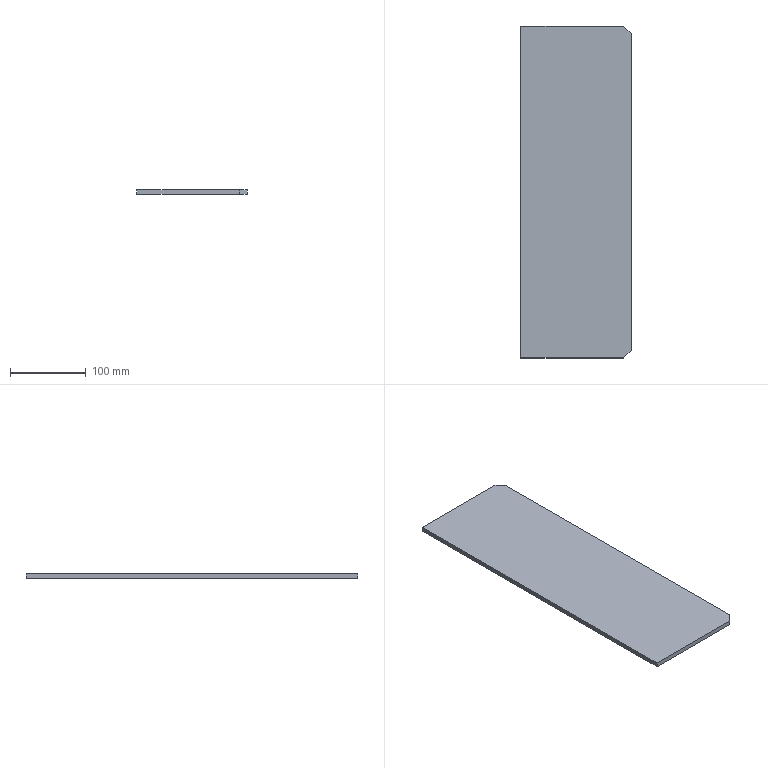Part | STEP file | 05-Rib plate 3 | 1 solid | 8 faces | box 146 x 439 x 6 mm | volume 383964 mm3 | plane 8
STEP:
#1=CARTESIAN_POINT('',(0.,0.,0.));
#2=DIRECTION('',(0.,0.,1.));
#3=DIRECTION('',(1.,0.,0.));
#4=AXIS2_PLACEMENT_3D('',#1,#2,#3);
#5=CARTESIAN_POINT('',(0.,0.,0.));
#6=VERTEX_POINT('',#5);
#7=CARTESIAN_POINT('',(0.,-439.,0.));
#8=VERTEX_POINT('',#7);
#9=CARTESIAN_POINT('',(0.,0.,0.));
#10=DIRECTION('',(0.,-1.,0.));
#11=VECTOR('',#10,1.);
#12=LINE('',#9,#11);
#13=CARTESIAN_POINT('',(0.,0.,6.));
#14=DIRECTION('',(1.,0.,0.));
#15=DIRECTION('',(0.,1.,0.));
#16=AXIS2_PLACEMENT_3D('',#13,#14,#15);
#17=PLANE('',#16);
#18=CARTESIAN_POINT('',(0.,-6.));
#19=DIRECTION('',(-1.,0.));
#20=VECTOR('',#19,1.);
#21=LINE('',#18,#20);
#22=(GEOMETRIC_REPRESENTATION_CONTEXT(2)PARAMETRIC_REPRESENTATION_CONTEXT()REPRESENTATION_CONTEXT('',''));
#23=DEFINITIONAL_REPRESENTATION('',(#21),#22);
#24=PCURVE('',#17,#23);
#25=CARTESIAN_POINT('',(0.,0.,0.));
#26=DIRECTION('',(0.,0.,1.));
#27=DIRECTION('',(1.,0.,0.));
#28=AXIS2_PLACEMENT_3D('',#25,#26,#27);
#29=PLANE('',#28);
#30=CARTESIAN_POINT('',(0.,0.));
#31=DIRECTION('',(0.,-1.));
#32=VECTOR('',#31,1.);
#33=LINE('',#30,#32);
#34=(GEOMETRIC_REPRESENTATION_CONTEXT(2)PARAMETRIC_REPRESENTATION_CONTEXT()REPRESENTATION_CONTEXT('',''));
#35=DEFINITIONAL_REPRESENTATION('',(#33),#34);
#36=PCURVE('',#29,#35);
#37=SURFACE_CURVE('',#12,(#24,#36),.PCURVE_S1.);
#38=EDGE_CURVE('',#6,#8,#37,.T.);
#39=ORIENTED_EDGE('',*,*,#38,.T.);
#40=CARTESIAN_POINT('',(0.,-439.,6.));
#41=VERTEX_POINT('',#40);
#42=CARTESIAN_POINT('',(0.,-439.,6.));
#43=DIRECTION('',(0.,0.,-1.));
#44=VECTOR('',#43,1.);
#45=LINE('',#42,#44);
#46=CARTESIAN_POINT('',(-439.,0.));
#47=DIRECTION('',(0.,-1.));
#48=VECTOR('',#47,1.);
#49=LINE('',#46,#48);
#50=(GEOMETRIC_REPRESENTATION_CONTEXT(2)PARAMETRIC_REPRESENTATION_CONTEXT()REPRESENTATION_CONTEXT('',''));
#51=DEFINITIONAL_REPRESENTATION('',(#49),#50);
#52=PCURVE('',#17,#51);
#53=CARTESIAN_POINT('',(0.,-439.,6.));
#54=DIRECTION('',(0.,1.,0.));
#55=DIRECTION('',(0.,0.,1.));
#56=AXIS2_PLACEMENT_3D('',#53,#54,#55);
#57=PLANE('',#56);
#58=CARTESIAN_POINT('',(0.,0.));
#59=DIRECTION('',(-1.,0.));
#60=VECTOR('',#59,1.);
#61=LINE('',#58,#60);
#62=(GEOMETRIC_REPRESENTATION_CONTEXT(2)PARAMETRIC_REPRESENTATION_CONTEXT()REPRESENTATION_CONTEXT('',''));
#63=DEFINITIONAL_REPRESENTATION('',(#61),#62);
#64=PCURVE('',#57,#63);
#65=SURFACE_CURVE('',#45,(#52,#64),.PCURVE_S1.);
#66=EDGE_CURVE('',#41,#8,#65,.T.);
#67=ORIENTED_EDGE('',*,*,#66,.F.);
#68=CARTESIAN_POINT('',(0.,0.,6.));
#69=VERTEX_POINT('',#68);
#70=CARTESIAN_POINT('',(0.,0.,6.));
#71=DIRECTION('',(0.,-1.,0.));
#72=VECTOR('',#71,1.);
#73=LINE('',#70,#72);
#74=CARTESIAN_POINT('',(0.,0.));
#75=DIRECTION('',(-1.,0.));
#76=VECTOR('',#75,1.);
#77=LINE('',#74,#76);
#78=(GEOMETRIC_REPRESENTATION_CONTEXT(2)PARAMETRIC_REPRESENTATION_CONTEXT()REPRESENTATION_CONTEXT('',''));
#79=DEFINITIONAL_REPRESENTATION('',(#77),#78);
#80=PCURVE('',#17,#79);
#81=CARTESIAN_POINT('',(0.,0.,6.));
#82=DIRECTION('',(0.,0.,1.));
#83=DIRECTION('',(1.,0.,0.));
#84=AXIS2_PLACEMENT_3D('',#81,#82,#83);
#85=PLANE('',#84);
#86=CARTESIAN_POINT('',(0.,0.));
#87=DIRECTION('',(0.,-1.));
#88=VECTOR('',#87,1.);
#89=LINE('',#86,#88);
#90=(GEOMETRIC_REPRESENTATION_CONTEXT(2)PARAMETRIC_REPRESENTATION_CONTEXT()REPRESENTATION_CONTEXT('',''));
#91=DEFINITIONAL_REPRESENTATION('',(#89),#90);
#92=PCURVE('',#85,#91);
#93=SURFACE_CURVE('',#73,(#80,#92),.PCURVE_S1.);
#94=EDGE_CURVE('',#69,#41,#93,.T.);
#95=ORIENTED_EDGE('',*,*,#94,.F.);
#96=CARTESIAN_POINT('',(0.,0.,6.));
#97=DIRECTION('',(0.,0.,-1.));
#98=VECTOR('',#97,1.);
#99=LINE('',#96,#98);
#100=CARTESIAN_POINT('',(0.,0.));
#101=DIRECTION('',(0.,-1.));
#102=VECTOR('',#101,1.);
#103=LINE('',#100,#102);
#104=(GEOMETRIC_REPRESENTATION_CONTEXT(2)PARAMETRIC_REPRESENTATION_CONTEXT()REPRESENTATION_CONTEXT('',''));
#105=DEFINITIONAL_REPRESENTATION('',(#103),#104);
#106=PCURVE('',#17,#105);
#107=CARTESIAN_POINT('',(0.,0.,6.));
#108=DIRECTION('',(0.,-1.,0.));
#109=DIRECTION('',(0.,0.,-1.));
#110=AXIS2_PLACEMENT_3D('',#107,#108,#109);
#111=PLANE('',#110);
#112=CARTESIAN_POINT('',(0.,0.));
#113=DIRECTION('',(1.,0.));
#114=VECTOR('',#113,1.);
#115=LINE('',#112,#114);
#116=(GEOMETRIC_REPRESENTATION_CONTEXT(2)PARAMETRIC_REPRESENTATION_CONTEXT()REPRESENTATION_CONTEXT('',''));
#117=DEFINITIONAL_REPRESENTATION('',(#115),#116);
#118=PCURVE('',#111,#117);
#119=SURFACE_CURVE('',#99,(#106,#118),.PCURVE_S1.);
#120=EDGE_CURVE('',#69,#6,#119,.T.);
#121=ORIENTED_EDGE('',*,*,#120,.T.);
#122=EDGE_LOOP('',(#39,#67,#95,#121));
#123=FACE_BOUND('',#122,.T.);
#124=ADVANCED_FACE('',(#123),#17,.F.);
#125=CARTESIAN_POINT('',(136.,-439.,0.));
#126=VERTEX_POINT('',#125);
#127=CARTESIAN_POINT('',(0.,-439.,0.));
#128=DIRECTION('',(1.,0.,0.));
#129=VECTOR('',#128,1.);
#130=LINE('',#127,#129);
#131=CARTESIAN_POINT('',(-6.,0.));
#132=DIRECTION('',(0.,1.));
#133=VECTOR('',#132,1.);
#134=LINE('',#131,#133);
#135=(GEOMETRIC_REPRESENTATION_CONTEXT(2)PARAMETRIC_REPRESENTATION_CONTEXT()REPRESENTATION_CONTEXT('',''));
#136=DEFINITIONAL_REPRESENTATION('',(#134),#135);
#137=PCURVE('',#57,#136);
#138=CARTESIAN_POINT('',(0.,-439.));
#139=DIRECTION('',(1.,0.));
#140=VECTOR('',#139,1.);
#141=LINE('',#138,#140);
#142=(GEOMETRIC_REPRESENTATION_CONTEXT(2)PARAMETRIC_REPRESENTATION_CONTEXT()REPRESENTATION_CONTEXT('',''));
#143=DEFINITIONAL_REPRESENTATION('',(#141),#142);
#144=PCURVE('',#29,#143);
#145=SURFACE_CURVE('',#130,(#137,#144),.PCURVE_S1.);
#146=EDGE_CURVE('',#8,#126,#145,.T.);
#147=ORIENTED_EDGE('',*,*,#146,.T.);
#148=CARTESIAN_POINT('',(136.,-439.,6.));
#149=VERTEX_POINT('',#148);
#150=CARTESIAN_POINT('',(136.,-439.,6.));
#151=DIRECTION('',(0.,0.,-1.));
#152=VECTOR('',#151,1.);
#153=LINE('',#150,#152);
#154=CARTESIAN_POINT('',(0.,136.));
#155=DIRECTION('',(-1.,0.));
#156=VECTOR('',#155,1.);
#157=LINE('',#154,#156);
#158=(GEOMETRIC_REPRESENTATION_CONTEXT(2)PARAMETRIC_REPRESENTATION_CONTEXT()REPRESENTATION_CONTEXT('',''));
#159=DEFINITIONAL_REPRESENTATION('',(#157),#158);
#160=PCURVE('',#57,#159);
#161=CARTESIAN_POINT('',(146.,-429.,6.));
#162=DIRECTION('',(-0.7071,0.7071,0.));
#163=DIRECTION('',(-0.7071,-0.7071,0.));
#164=AXIS2_PLACEMENT_3D('',#161,#162,#163);
#165=PLANE('',#164);
#166=CARTESIAN_POINT('',(14.142,0.));
#167=DIRECTION('',(0.,-1.));
#168=VECTOR('',#167,1.);
#169=LINE('',#166,#168);
#170=(GEOMETRIC_REPRESENTATION_CONTEXT(2)PARAMETRIC_REPRESENTATION_CONTEXT()REPRESENTATION_CONTEXT('',''));
#171=DEFINITIONAL_REPRESENTATION('',(#169),#170);
#172=PCURVE('',#165,#171);
#173=SURFACE_CURVE('',#153,(#160,#172),.PCURVE_S1.);
#174=EDGE_CURVE('',#149,#126,#173,.T.);
#175=ORIENTED_EDGE('',*,*,#174,.F.);
#176=CARTESIAN_POINT('',(0.,-439.,6.));
#177=DIRECTION('',(1.,0.,0.));
#178=VECTOR('',#177,1.);
#179=LINE('',#176,#178);
#180=CARTESIAN_POINT('',(0.,0.));
#181=DIRECTION('',(0.,1.));
#182=VECTOR('',#181,1.);
#183=LINE('',#180,#182);
#184=(GEOMETRIC_REPRESENTATION_CONTEXT(2)PARAMETRIC_REPRESENTATION_CONTEXT()REPRESENTATION_CONTEXT('',''));
#185=DEFINITIONAL_REPRESENTATION('',(#183),#184);
#186=PCURVE('',#57,#185);
#187=CARTESIAN_POINT('',(0.,-439.));
#188=DIRECTION('',(1.,0.));
#189=VECTOR('',#188,1.);
#190=LINE('',#187,#189);
#191=(GEOMETRIC_REPRESENTATION_CONTEXT(2)PARAMETRIC_REPRESENTATION_CONTEXT()REPRESENTATION_CONTEXT('',''));
#192=DEFINITIONAL_REPRESENTATION('',(#190),#191);
#193=PCURVE('',#85,#192);
#194=SURFACE_CURVE('',#179,(#186,#193),.PCURVE_S1.);
#195=EDGE_CURVE('',#41,#149,#194,.T.);
#196=ORIENTED_EDGE('',*,*,#195,.F.);
#197=ORIENTED_EDGE('',*,*,#66,.T.);
#198=EDGE_LOOP('',(#147,#175,#196,#197));
#199=FACE_BOUND('',#198,.T.);
#200=ADVANCED_FACE('',(#199),#57,.F.);
#201=CARTESIAN_POINT('',(146.,-429.,0.));
#202=VERTEX_POINT('',#201);
#203=CARTESIAN_POINT('',(146.,-429.,0.));
#204=DIRECTION('',(0.7071,0.7071,0.));
#205=VECTOR('',#204,1.);
#206=LINE('',#203,#205);
#207=CARTESIAN_POINT('',(0.,-6.));
#208=DIRECTION('',(-1.,0.));
#209=VECTOR('',#208,1.);
#210=LINE('',#207,#209);
#211=(GEOMETRIC_REPRESENTATION_CONTEXT(2)PARAMETRIC_REPRESENTATION_CONTEXT()REPRESENTATION_CONTEXT('',''));
#212=DEFINITIONAL_REPRESENTATION('',(#210),#211);
#213=PCURVE('',#165,#212);
#214=CARTESIAN_POINT('',(146.,-429.));
#215=DIRECTION('',(0.7071,0.7071));
#216=VECTOR('',#215,1.);
#217=LINE('',#214,#216);
#218=(GEOMETRIC_REPRESENTATION_CONTEXT(2)PARAMETRIC_REPRESENTATION_CONTEXT()REPRESENTATION_CONTEXT('',''));
#219=DEFINITIONAL_REPRESENTATION('',(#217),#218);
#220=PCURVE('',#29,#219);
#221=SURFACE_CURVE('',#206,(#213,#220),.PCURVE_S1.);
#222=EDGE_CURVE('',#126,#202,#221,.T.);
#223=ORIENTED_EDGE('',*,*,#222,.T.);
#224=CARTESIAN_POINT('',(146.,-429.,6.));
#225=VERTEX_POINT('',#224);
#226=CARTESIAN_POINT('',(146.,-429.,6.));
#227=DIRECTION('',(0.,0.,-1.));
#228=VECTOR('',#227,1.);
#229=LINE('',#226,#228);
#230=CARTESIAN_POINT('',(0.,0.));
#231=DIRECTION('',(0.,-1.));
#232=VECTOR('',#231,1.);
#233=LINE('',#230,#232);
#234=(GEOMETRIC_REPRESENTATION_CONTEXT(2)PARAMETRIC_REPRESENTATION_CONTEXT()REPRESENTATION_CONTEXT('',''));
#235=DEFINITIONAL_REPRESENTATION('',(#233),#234);
#236=PCURVE('',#165,#235);
#237=CARTESIAN_POINT('',(146.,-10.,6.));
#238=DIRECTION('',(-1.,0.,0.));
#239=DIRECTION('',(0.,-1.,0.));
#240=AXIS2_PLACEMENT_3D('',#237,#238,#239);
#241=PLANE('',#240);
#242=CARTESIAN_POINT('',(419.,0.));
#243=DIRECTION('',(0.,-1.));
#244=VECTOR('',#243,1.);
#245=LINE('',#242,#244);
#246=(GEOMETRIC_REPRESENTATION_CONTEXT(2)PARAMETRIC_REPRESENTATION_CONTEXT()REPRESENTATION_CONTEXT('',''));
#247=DEFINITIONAL_REPRESENTATION('',(#245),#246);
#248=PCURVE('',#241,#247);
#249=SURFACE_CURVE('',#229,(#236,#248),.PCURVE_S1.);
#250=EDGE_CURVE('',#225,#202,#249,.T.);
#251=ORIENTED_EDGE('',*,*,#250,.F.);
#252=CARTESIAN_POINT('',(146.,-429.,6.));
#253=DIRECTION('',(0.7071,0.7071,0.));
#254=VECTOR('',#253,1.);
#255=LINE('',#252,#254);
#256=CARTESIAN_POINT('',(0.,0.));
#257=DIRECTION('',(-1.,0.));
#258=VECTOR('',#257,1.);
#259=LINE('',#256,#258);
#260=(GEOMETRIC_REPRESENTATION_CONTEXT(2)PARAMETRIC_REPRESENTATION_CONTEXT()REPRESENTATION_CONTEXT('',''));
#261=DEFINITIONAL_REPRESENTATION('',(#259),#260);
#262=PCURVE('',#165,#261);
#263=CARTESIAN_POINT('',(146.,-429.));
#264=DIRECTION('',(0.7071,0.7071));
#265=VECTOR('',#264,1.);
#266=LINE('',#263,#265);
#267=(GEOMETRIC_REPRESENTATION_CONTEXT(2)PARAMETRIC_REPRESENTATION_CONTEXT()REPRESENTATION_CONTEXT('',''));
#268=DEFINITIONAL_REPRESENTATION('',(#266),#267);
#269=PCURVE('',#85,#268);
#270=SURFACE_CURVE('',#255,(#262,#269),.PCURVE_S1.);
#271=EDGE_CURVE('',#149,#225,#270,.T.);
#272=ORIENTED_EDGE('',*,*,#271,.F.);
#273=ORIENTED_EDGE('',*,*,#174,.T.);
#274=EDGE_LOOP('',(#223,#251,#272,#273));
#275=FACE_BOUND('',#274,.T.);
#276=ADVANCED_FACE('',(#275),#165,.F.);
#277=CARTESIAN_POINT('',(146.,-10.,0.));
#278=VERTEX_POINT('',#277);
#279=CARTESIAN_POINT('',(146.,-10.,0.));
#280=DIRECTION('',(0.,1.,0.));
#281=VECTOR('',#280,1.);
#282=LINE('',#279,#281);
#283=CARTESIAN_POINT('',(0.,-6.));
#284=DIRECTION('',(-1.,0.));
#285=VECTOR('',#284,1.);
#286=LINE('',#283,#285);
#287=(GEOMETRIC_REPRESENTATION_CONTEXT(2)PARAMETRIC_REPRESENTATION_CONTEXT()REPRESENTATION_CONTEXT('',''));
#288=DEFINITIONAL_REPRESENTATION('',(#286),#287);
#289=PCURVE('',#241,#288);
#290=CARTESIAN_POINT('',(146.,-10.));
#291=DIRECTION('',(0.,1.));
#292=VECTOR('',#291,1.);
#293=LINE('',#290,#292);
#294=(GEOMETRIC_REPRESENTATION_CONTEXT(2)PARAMETRIC_REPRESENTATION_CONTEXT()REPRESENTATION_CONTEXT('',''));
#295=DEFINITIONAL_REPRESENTATION('',(#293),#294);
#296=PCURVE('',#29,#295);
#297=SURFACE_CURVE('',#282,(#289,#296),.PCURVE_S1.);
#298=EDGE_CURVE('',#202,#278,#297,.T.);
#299=ORIENTED_EDGE('',*,*,#298,.T.);
#300=CARTESIAN_POINT('',(146.,-10.,6.));
#301=VERTEX_POINT('',#300);
#302=CARTESIAN_POINT('',(146.,-10.,6.));
#303=DIRECTION('',(0.,0.,-1.));
#304=VECTOR('',#303,1.);
#305=LINE('',#302,#304);
#306=CARTESIAN_POINT('',(0.,0.));
#307=DIRECTION('',(0.,-1.));
#308=VECTOR('',#307,1.);
#309=LINE('',#306,#308);
#310=(GEOMETRIC_REPRESENTATION_CONTEXT(2)PARAMETRIC_REPRESENTATION_CONTEXT()REPRESENTATION_CONTEXT('',''));
#311=DEFINITIONAL_REPRESENTATION('',(#309),#310);
#312=PCURVE('',#241,#311);
#313=CARTESIAN_POINT('',(136.,0.,6.));
#314=DIRECTION('',(-0.7071,-0.7071,0.));
#315=DIRECTION('',(0.7071,-0.7071,0.));
#316=AXIS2_PLACEMENT_3D('',#313,#314,#315);
#317=PLANE('',#316);
#318=CARTESIAN_POINT('',(14.142,0.));
#319=DIRECTION('',(0.,-1.));
#320=VECTOR('',#319,1.);
#321=LINE('',#318,#320);
#322=(GEOMETRIC_REPRESENTATION_CONTEXT(2)PARAMETRIC_REPRESENTATION_CONTEXT()REPRESENTATION_CONTEXT('',''));
#323=DEFINITIONAL_REPRESENTATION('',(#321),#322);
#324=PCURVE('',#317,#323);
#325=SURFACE_CURVE('',#305,(#312,#324),.PCURVE_S1.);
#326=EDGE_CURVE('',#301,#278,#325,.T.);
#327=ORIENTED_EDGE('',*,*,#326,.F.);
#328=CARTESIAN_POINT('',(146.,-10.,6.));
#329=DIRECTION('',(0.,1.,0.));
#330=VECTOR('',#329,1.);
#331=LINE('',#328,#330);
#332=CARTESIAN_POINT('',(0.,0.));
#333=DIRECTION('',(-1.,0.));
#334=VECTOR('',#333,1.);
#335=LINE('',#332,#334);
#336=(GEOMETRIC_REPRESENTATION_CONTEXT(2)PARAMETRIC_REPRESENTATION_CONTEXT()REPRESENTATION_CONTEXT('',''));
#337=DEFINITIONAL_REPRESENTATION('',(#335),#336);
#338=PCURVE('',#241,#337);
#339=CARTESIAN_POINT('',(146.,-10.));
#340=DIRECTION('',(0.,1.));
#341=VECTOR('',#340,1.);
#342=LINE('',#339,#341);
#343=(GEOMETRIC_REPRESENTATION_CONTEXT(2)PARAMETRIC_REPRESENTATION_CONTEXT()REPRESENTATION_CONTEXT('',''));
#344=DEFINITIONAL_REPRESENTATION('',(#342),#343);
#345=PCURVE('',#85,#344);
#346=SURFACE_CURVE('',#331,(#338,#345),.PCURVE_S1.);
#347=EDGE_CURVE('',#225,#301,#346,.T.);
#348=ORIENTED_EDGE('',*,*,#347,.F.);
#349=ORIENTED_EDGE('',*,*,#250,.T.);
#350=EDGE_LOOP('',(#299,#327,#348,#349));
#351=FACE_BOUND('',#350,.T.);
#352=ADVANCED_FACE('',(#351),#241,.F.);
#353=CARTESIAN_POINT('',(136.,0.,0.));
#354=VERTEX_POINT('',#353);
#355=CARTESIAN_POINT('',(136.,0.,0.));
#356=DIRECTION('',(-0.7071,0.7071,0.));
#357=VECTOR('',#356,1.);
#358=LINE('',#355,#357);
#359=CARTESIAN_POINT('',(0.,-6.));
#360=DIRECTION('',(-1.,0.));
#361=VECTOR('',#360,1.);
#362=LINE('',#359,#361);
#363=(GEOMETRIC_REPRESENTATION_CONTEXT(2)PARAMETRIC_REPRESENTATION_CONTEXT()REPRESENTATION_CONTEXT('',''));
#364=DEFINITIONAL_REPRESENTATION('',(#362),#363);
#365=PCURVE('',#317,#364);
#366=CARTESIAN_POINT('',(136.,0.));
#367=DIRECTION('',(-0.7071,0.7071));
#368=VECTOR('',#367,1.);
#369=LINE('',#366,#368);
#370=(GEOMETRIC_REPRESENTATION_CONTEXT(2)PARAMETRIC_REPRESENTATION_CONTEXT()REPRESENTATION_CONTEXT('',''));
#371=DEFINITIONAL_REPRESENTATION('',(#369),#370);
#372=PCURVE('',#29,#371);
#373=SURFACE_CURVE('',#358,(#365,#372),.PCURVE_S1.);
#374=EDGE_CURVE('',#278,#354,#373,.T.);
#375=ORIENTED_EDGE('',*,*,#374,.T.);
#376=CARTESIAN_POINT('',(136.,0.,6.));
#377=VERTEX_POINT('',#376);
#378=CARTESIAN_POINT('',(136.,0.,6.));
#379=DIRECTION('',(0.,0.,-1.));
#380=VECTOR('',#379,1.);
#381=LINE('',#378,#380);
#382=CARTESIAN_POINT('',(0.,0.));
#383=DIRECTION('',(0.,-1.));
#384=VECTOR('',#383,1.);
#385=LINE('',#382,#384);
#386=(GEOMETRIC_REPRESENTATION_CONTEXT(2)PARAMETRIC_REPRESENTATION_CONTEXT()REPRESENTATION_CONTEXT('',''));
#387=DEFINITIONAL_REPRESENTATION('',(#385),#386);
#388=PCURVE('',#317,#387);
#389=CARTESIAN_POINT('',(0.,136.));
#390=DIRECTION('',(1.,0.));
#391=VECTOR('',#390,1.);
#392=LINE('',#389,#391);
#393=(GEOMETRIC_REPRESENTATION_CONTEXT(2)PARAMETRIC_REPRESENTATION_CONTEXT()REPRESENTATION_CONTEXT('',''));
#394=DEFINITIONAL_REPRESENTATION('',(#392),#393);
#395=PCURVE('',#111,#394);
#396=SURFACE_CURVE('',#381,(#388,#395),.PCURVE_S1.);
#397=EDGE_CURVE('',#377,#354,#396,.T.);
#398=ORIENTED_EDGE('',*,*,#397,.F.);
#399=CARTESIAN_POINT('',(136.,0.,6.));
#400=DIRECTION('',(-0.7071,0.7071,0.));
#401=VECTOR('',#400,1.);
#402=LINE('',#399,#401);
#403=CARTESIAN_POINT('',(0.,0.));
#404=DIRECTION('',(-1.,0.));
#405=VECTOR('',#404,1.);
#406=LINE('',#403,#405);
#407=(GEOMETRIC_REPRESENTATION_CONTEXT(2)PARAMETRIC_REPRESENTATION_CONTEXT()REPRESENTATION_CONTEXT('',''));
#408=DEFINITIONAL_REPRESENTATION('',(#406),#407);
#409=PCURVE('',#317,#408);
#410=CARTESIAN_POINT('',(136.,0.));
#411=DIRECTION('',(-0.7071,0.7071));
#412=VECTOR('',#411,1.);
#413=LINE('',#410,#412);
#414=(GEOMETRIC_REPRESENTATION_CONTEXT(2)PARAMETRIC_REPRESENTATION_CONTEXT()REPRESENTATION_CONTEXT('',''));
#415=DEFINITIONAL_REPRESENTATION('',(#413),#414);
#416=PCURVE('',#85,#415);
#417=SURFACE_CURVE('',#402,(#409,#416),.PCURVE_S1.);
#418=EDGE_CURVE('',#301,#377,#417,.T.);
#419=ORIENTED_EDGE('',*,*,#418,.F.);
#420=ORIENTED_EDGE('',*,*,#326,.T.);
#421=EDGE_LOOP('',(#375,#398,#419,#420));
#422=FACE_BOUND('',#421,.T.);
#423=ADVANCED_FACE('',(#422),#317,.F.);
#424=CARTESIAN_POINT('',(0.,0.,0.));
#425=DIRECTION('',(-1.,0.,0.));
#426=VECTOR('',#425,1.);
#427=LINE('',#424,#426);
#428=CARTESIAN_POINT('',(6.,0.));
#429=DIRECTION('',(0.,-1.));
#430=VECTOR('',#429,1.);
#431=LINE('',#428,#430);
#432=(GEOMETRIC_REPRESENTATION_CONTEXT(2)PARAMETRIC_REPRESENTATION_CONTEXT()REPRESENTATION_CONTEXT('',''));
#433=DEFINITIONAL_REPRESENTATION('',(#431),#432);
#434=PCURVE('',#111,#433);
#435=CARTESIAN_POINT('',(0.,0.));
#436=DIRECTION('',(-1.,0.));
#437=VECTOR('',#436,1.);
#438=LINE('',#435,#437);
#439=(GEOMETRIC_REPRESENTATION_CONTEXT(2)PARAMETRIC_REPRESENTATION_CONTEXT()REPRESENTATION_CONTEXT('',''));
#440=DEFINITIONAL_REPRESENTATION('',(#438),#439);
#441=PCURVE('',#29,#440);
#442=SURFACE_CURVE('',#427,(#434,#441),.PCURVE_S1.);
#443=EDGE_CURVE('',#354,#6,#442,.T.);
#444=ORIENTED_EDGE('',*,*,#443,.T.);
#445=ORIENTED_EDGE('',*,*,#120,.F.);
#446=CARTESIAN_POINT('',(0.,0.,6.));
#447=DIRECTION('',(-1.,0.,0.));
#448=VECTOR('',#447,1.);
#449=LINE('',#446,#448);
#450=CARTESIAN_POINT('',(0.,0.));
#451=DIRECTION('',(0.,-1.));
#452=VECTOR('',#451,1.);
#453=LINE('',#450,#452);
#454=(GEOMETRIC_REPRESENTATION_CONTEXT(2)PARAMETRIC_REPRESENTATION_CONTEXT()REPRESENTATION_CONTEXT('',''));
#455=DEFINITIONAL_REPRESENTATION('',(#453),#454);
#456=PCURVE('',#111,#455);
#457=CARTESIAN_POINT('',(0.,0.));
#458=DIRECTION('',(-1.,0.));
#459=VECTOR('',#458,1.);
#460=LINE('',#457,#459);
#461=(GEOMETRIC_REPRESENTATION_CONTEXT(2)PARAMETRIC_REPRESENTATION_CONTEXT()REPRESENTATION_CONTEXT('',''));
#462=DEFINITIONAL_REPRESENTATION('',(#460),#461);
#463=PCURVE('',#85,#462);
#464=SURFACE_CURVE('',#449,(#456,#463),.PCURVE_S1.);
#465=EDGE_CURVE('',#377,#69,#464,.T.);
#466=ORIENTED_EDGE('',*,*,#465,.F.);
#467=ORIENTED_EDGE('',*,*,#397,.T.);
#468=EDGE_LOOP('',(#444,#445,#466,#467));
#469=FACE_BOUND('',#468,.T.);
#470=ADVANCED_FACE('',(#469),#111,.F.);
#471=ORIENTED_EDGE('',*,*,#94,.T.);
#472=ORIENTED_EDGE('',*,*,#195,.T.);
#473=ORIENTED_EDGE('',*,*,#271,.T.);
#474=ORIENTED_EDGE('',*,*,#347,.T.);
#475=ORIENTED_EDGE('',*,*,#418,.T.);
#476=ORIENTED_EDGE('',*,*,#465,.T.);
#477=EDGE_LOOP('',(#471,#472,#473,#474,#475,#476));
#478=FACE_BOUND('',#477,.T.);
#479=ADVANCED_FACE('',(#478),#85,.T.);
#480=ORIENTED_EDGE('',*,*,#38,.F.);
#481=ORIENTED_EDGE('',*,*,#443,.F.);
#482=ORIENTED_EDGE('',*,*,#374,.F.);
#483=ORIENTED_EDGE('',*,*,#298,.F.);
#484=ORIENTED_EDGE('',*,*,#222,.F.);
#485=ORIENTED_EDGE('',*,*,#146,.F.);
#486=EDGE_LOOP('',(#480,#481,#482,#483,#484,#485));
#487=FACE_BOUND('',#486,.T.);
#488=ADVANCED_FACE('',(#487),#29,.F.);
#489=CLOSED_SHELL('',(#124,#200,#276,#352,#423,#470,#479,#488));
#490=MANIFOLD_SOLID_BREP('',#489);
#491=(LENGTH_UNIT()NAMED_UNIT(*)SI_UNIT(.MILLI.,.METRE.));
#492=UNCERTAINTY_MEASURE_WITH_UNIT(LENGTH_MEASURE(0.0000001),#491,'','');
#493=(NAMED_UNIT(*)PLANE_ANGLE_UNIT()SI_UNIT($,.RADIAN.));
#494=(NAMED_UNIT(*)SI_UNIT($,.STERADIAN.)SOLID_ANGLE_UNIT());
#495=(GEOMETRIC_REPRESENTATION_CONTEXT(3)GLOBAL_UNCERTAINTY_ASSIGNED_CONTEXT((#492))GLOBAL_UNIT_ASSIGNED_CONTEXT((#491,#493,#494))REPRESENTATION_CONTEXT('',''));
#496=ADVANCED_BREP_SHAPE_REPRESENTATION('',(#4,#490),#495);